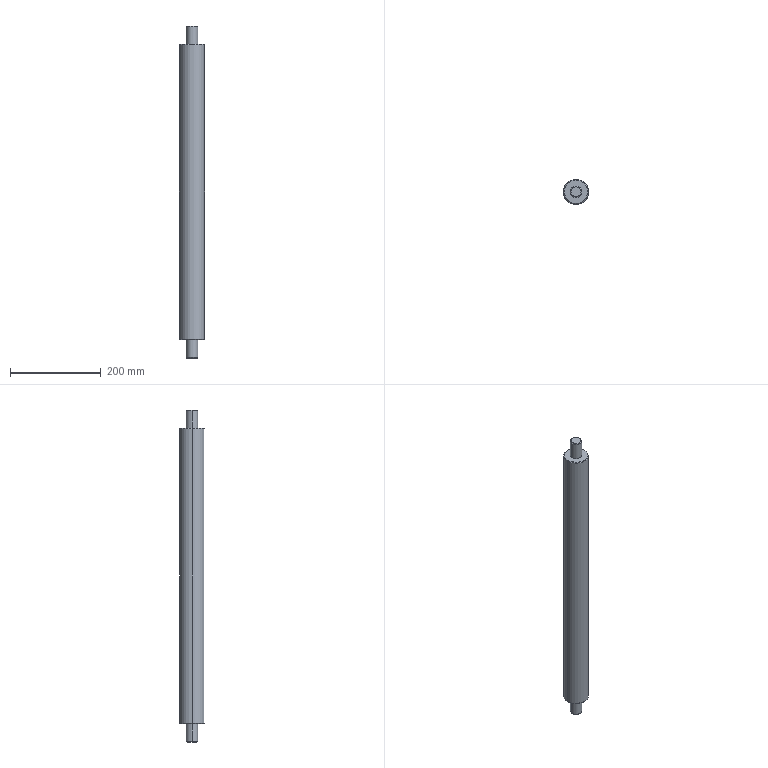Part | SolidWorks | features Chamfer 1, Extrusion 1, ICE 1, MirrorPattern 1 | 1 solid | 18 faces | box 55 x 55 x 730 mm | volume 1583008 mm3 | cone 8 | cylinder 6 | plane 4 | commonest cylinder face diameters 25 x4 55 x2
STEP:
#1=CARTESIAN_POINT('',(26.,0.,325.));
#2=VERTEX_POINT('',#1);
#3=CARTESIAN_POINT('',(-26.,0.,325.));
#4=VERTEX_POINT('',#3);
#5=CARTESIAN_POINT('',(0.,0.,325.));
#6=DIRECTION('',(0.,0.,1.));
#7=DIRECTION('',(1.,0.,0.));
#8=AXIS2_PLACEMENT_3D('',#5,#6,#7);
#9=CIRCLE('',#8,26.);
#10=EDGE_CURVE('',#2,#4,#9,.T.);
#11=ORIENTED_EDGE('',*,*,#10,.F.);
#12=CARTESIAN_POINT('',(27.5,0.,323.5));
#13=VERTEX_POINT('',#12);
#14=CARTESIAN_POINT('',(26.,0.,325.));
#15=DIRECTION('',(0.7071,0.,-0.7071));
#16=VECTOR('',#15,1000.);
#17=LINE('',#14,#16);
#18=EDGE_CURVE('',#2,#13,#17,.T.);
#19=ORIENTED_EDGE('',*,*,#18,.T.);
#20=CARTESIAN_POINT('',(-27.5,0.,323.5));
#21=VERTEX_POINT('',#20);
#22=CARTESIAN_POINT('',(0.,0.,323.5));
#23=DIRECTION('',(0.,0.,-1.));
#24=DIRECTION('',(1.,0.,0.));
#25=AXIS2_PLACEMENT_3D('',#22,#23,#24);
#26=CIRCLE('',#25,27.5);
#27=EDGE_CURVE('',#21,#13,#26,.T.);
#28=ORIENTED_EDGE('',*,*,#27,.F.);
#29=CARTESIAN_POINT('',(-26.,0.,325.));
#30=DIRECTION('',(-0.7071,0.,-0.7071));
#31=VECTOR('',#30,1000.);
#32=LINE('',#29,#31);
#33=EDGE_CURVE('',#4,#21,#32,.T.);
#34=ORIENTED_EDGE('',*,*,#33,.F.);
#35=EDGE_LOOP('',(#11,#19,#28,#34));
#36=FACE_OUTER_BOUND('',#35,.T.);
#37=CARTESIAN_POINT('',(0.,0.,325.));
#38=DIRECTION('',(0.,0.,-1.));
#39=DIRECTION('',(-1.,0.,0.));
#40=AXIS2_PLACEMENT_3D('',#37,#38,#39);
#41=CONICAL_SURFACE('',#40,26.,0.7854);
#42=ADVANCED_FACE('',(#36),#41,.T.);
#43=CARTESIAN_POINT('',(11.,0.,365.));
#44=VERTEX_POINT('',#43);
#45=CARTESIAN_POINT('',(-11.,0.,365.));
#46=VERTEX_POINT('',#45);
#47=CARTESIAN_POINT('',(0.,0.,365.));
#48=DIRECTION('',(0.,0.,1.));
#49=DIRECTION('',(1.,0.,0.));
#50=AXIS2_PLACEMENT_3D('',#47,#48,#49);
#51=CIRCLE('',#50,11.);
#52=EDGE_CURVE('',#44,#46,#51,.T.);
#53=ORIENTED_EDGE('',*,*,#52,.F.);
#54=CARTESIAN_POINT('',(12.5,0.,363.5));
#55=VERTEX_POINT('',#54);
#56=CARTESIAN_POINT('',(11.,0.,365.));
#57=DIRECTION('',(0.7071,0.,-0.7071));
#58=VECTOR('',#57,1000.);
#59=LINE('',#56,#58);
#60=EDGE_CURVE('',#44,#55,#59,.T.);
#61=ORIENTED_EDGE('',*,*,#60,.T.);
#62=CARTESIAN_POINT('',(-12.5,0.,363.5));
#63=VERTEX_POINT('',#62);
#64=CARTESIAN_POINT('',(0.,0.,363.5));
#65=DIRECTION('',(0.,0.,-1.));
#66=DIRECTION('',(1.,0.,0.));
#67=AXIS2_PLACEMENT_3D('',#64,#65,#66);
#68=CIRCLE('',#67,12.5);
#69=EDGE_CURVE('',#63,#55,#68,.T.);
#70=ORIENTED_EDGE('',*,*,#69,.F.);
#71=CARTESIAN_POINT('',(-11.,0.,365.));
#72=DIRECTION('',(-0.7071,0.,-0.7071));
#73=VECTOR('',#72,1000.);
#74=LINE('',#71,#73);
#75=EDGE_CURVE('',#46,#63,#74,.T.);
#76=ORIENTED_EDGE('',*,*,#75,.F.);
#77=EDGE_LOOP('',(#53,#61,#70,#76));
#78=FACE_OUTER_BOUND('',#77,.T.);
#79=CARTESIAN_POINT('',(0.,0.,365.));
#80=DIRECTION('',(0.,0.,-1.));
#81=DIRECTION('',(-1.,0.,0.));
#82=AXIS2_PLACEMENT_3D('',#79,#80,#81);
#83=CONICAL_SURFACE('',#82,11.,0.7854);
#84=ADVANCED_FACE('',(#78),#83,.T.);
#85=CARTESIAN_POINT('',(-26.,0.,-325.));
#86=VERTEX_POINT('',#85);
#87=CARTESIAN_POINT('',(26.,0.,-325.));
#88=VERTEX_POINT('',#87);
#89=CARTESIAN_POINT('',(0.,0.,-325.));
#90=DIRECTION('',(0.,0.,-1.));
#91=DIRECTION('',(1.,0.,0.));
#92=AXIS2_PLACEMENT_3D('',#89,#90,#91);
#93=CIRCLE('',#92,26.);
#94=EDGE_CURVE('',#86,#88,#93,.T.);
#95=ORIENTED_EDGE('',*,*,#94,.F.);
#96=CARTESIAN_POINT('',(-27.5,0.,-323.5));
#97=VERTEX_POINT('',#96);
#98=CARTESIAN_POINT('',(-27.5,0.,-323.5));
#99=DIRECTION('',(-0.7071,0.,0.7071));
#100=VECTOR('',#99,1000.);
#101=LINE('',#98,#100);
#102=EDGE_CURVE('',#86,#97,#101,.T.);
#103=ORIENTED_EDGE('',*,*,#102,.T.);
#104=CARTESIAN_POINT('',(27.5,0.,-323.5));
#105=VERTEX_POINT('',#104);
#106=CARTESIAN_POINT('',(0.,0.,-323.5));
#107=DIRECTION('',(0.,0.,1.));
#108=DIRECTION('',(1.,0.,0.));
#109=AXIS2_PLACEMENT_3D('',#106,#107,#108);
#110=CIRCLE('',#109,27.5);
#111=EDGE_CURVE('',#105,#97,#110,.T.);
#112=ORIENTED_EDGE('',*,*,#111,.F.);
#113=CARTESIAN_POINT('',(27.5,0.,-323.5));
#114=DIRECTION('',(0.7071,0.,0.7071));
#115=VECTOR('',#114,1000.);
#116=LINE('',#113,#115);
#117=EDGE_CURVE('',#88,#105,#116,.T.);
#118=ORIENTED_EDGE('',*,*,#117,.F.);
#119=EDGE_LOOP('',(#95,#103,#112,#118));
#120=FACE_OUTER_BOUND('',#119,.T.);
#121=CARTESIAN_POINT('',(0.,0.,-323.5));
#122=DIRECTION('',(0.,0.,1.));
#123=DIRECTION('',(1.,0.,0.));
#124=AXIS2_PLACEMENT_3D('',#121,#122,#123);
#125=CONICAL_SURFACE('',#124,27.5,0.7854);
#126=ADVANCED_FACE('',(#120),#125,.T.);
#127=CARTESIAN_POINT('',(-11.,0.,-365.));
#128=VERTEX_POINT('',#127);
#129=CARTESIAN_POINT('',(11.,0.,-365.));
#130=VERTEX_POINT('',#129);
#131=CARTESIAN_POINT('',(0.,0.,-365.));
#132=DIRECTION('',(0.,0.,-1.));
#133=DIRECTION('',(-1.,0.,0.));
#134=AXIS2_PLACEMENT_3D('',#131,#132,#133);
#135=CIRCLE('',#134,11.);
#136=EDGE_CURVE('',#128,#130,#135,.T.);
#137=ORIENTED_EDGE('',*,*,#136,.F.);
#138=CARTESIAN_POINT('',(-12.5,0.,-363.5));
#139=VERTEX_POINT('',#138);
#140=CARTESIAN_POINT('',(-12.5,0.,-363.5));
#141=DIRECTION('',(-0.7071,0.,0.7071));
#142=VECTOR('',#141,1000.);
#143=LINE('',#140,#142);
#144=EDGE_CURVE('',#128,#139,#143,.T.);
#145=ORIENTED_EDGE('',*,*,#144,.T.);
#146=CARTESIAN_POINT('',(12.5,0.,-363.5));
#147=VERTEX_POINT('',#146);
#148=CARTESIAN_POINT('',(0.,0.,-363.5));
#149=DIRECTION('',(0.,0.,1.));
#150=DIRECTION('',(-1.,0.,0.));
#151=AXIS2_PLACEMENT_3D('',#148,#149,#150);
#152=CIRCLE('',#151,12.5);
#153=EDGE_CURVE('',#147,#139,#152,.T.);
#154=ORIENTED_EDGE('',*,*,#153,.F.);
#155=CARTESIAN_POINT('',(12.5,0.,-363.5));
#156=DIRECTION('',(0.7071,0.,0.7071));
#157=VECTOR('',#156,1000.);
#158=LINE('',#155,#157);
#159=EDGE_CURVE('',#130,#147,#158,.T.);
#160=ORIENTED_EDGE('',*,*,#159,.F.);
#161=EDGE_LOOP('',(#137,#145,#154,#160));
#162=FACE_OUTER_BOUND('',#161,.T.);
#163=CARTESIAN_POINT('',(0.,0.,-363.5));
#164=DIRECTION('',(0.,0.,1.));
#165=DIRECTION('',(1.,0.,0.));
#166=AXIS2_PLACEMENT_3D('',#163,#164,#165);
#167=CONICAL_SURFACE('',#166,12.5,0.7854);
#168=ADVANCED_FACE('',(#162),#167,.T.);
#169=ORIENTED_EDGE('',*,*,#153,.T.);
#170=CARTESIAN_POINT('',(-12.5,0.,-325.));
#171=VERTEX_POINT('',#170);
#172=CARTESIAN_POINT('',(-12.5,0.,-365.));
#173=DIRECTION('',(0.,0.,1.));
#174=VECTOR('',#173,1000.);
#175=LINE('',#172,#174);
#176=EDGE_CURVE('',#139,#171,#175,.T.);
#177=ORIENTED_EDGE('',*,*,#176,.T.);
#178=CARTESIAN_POINT('',(12.5,0.,-325.));
#179=VERTEX_POINT('',#178);
#180=CARTESIAN_POINT('',(0.,0.,-325.));
#181=DIRECTION('',(0.,0.,1.));
#182=DIRECTION('',(1.,0.,0.));
#183=AXIS2_PLACEMENT_3D('',#180,#181,#182);
#184=CIRCLE('',#183,12.5);
#185=EDGE_CURVE('',#179,#171,#184,.T.);
#186=ORIENTED_EDGE('',*,*,#185,.F.);
#187=CARTESIAN_POINT('',(12.5,0.,-365.));
#188=DIRECTION('',(0.,0.,1.));
#189=VECTOR('',#188,1000.);
#190=LINE('',#187,#189);
#191=EDGE_CURVE('',#147,#179,#190,.T.);
#192=ORIENTED_EDGE('',*,*,#191,.F.);
#193=EDGE_LOOP('',(#169,#177,#186,#192));
#194=FACE_OUTER_BOUND('',#193,.T.);
#195=CARTESIAN_POINT('',(0.,0.,-365.));
#196=DIRECTION('',(0.,0.,1.));
#197=DIRECTION('',(1.,0.,0.));
#198=AXIS2_PLACEMENT_3D('',#195,#196,#197);
#199=CYLINDRICAL_SURFACE('',#198,12.5);
#200=ADVANCED_FACE('',(#194),#199,.T.);
#201=ORIENTED_EDGE('',*,*,#69,.T.);
#202=CARTESIAN_POINT('',(12.5,0.,325.));
#203=VERTEX_POINT('',#202);
#204=CARTESIAN_POINT('',(12.5,0.,365.));
#205=DIRECTION('',(0.,0.,-1.));
#206=VECTOR('',#205,1000.);
#207=LINE('',#204,#206);
#208=EDGE_CURVE('',#55,#203,#207,.T.);
#209=ORIENTED_EDGE('',*,*,#208,.T.);
#210=CARTESIAN_POINT('',(-12.5,0.,325.));
#211=VERTEX_POINT('',#210);
#212=CARTESIAN_POINT('',(0.,0.,325.));
#213=DIRECTION('',(0.,0.,1.));
#214=DIRECTION('',(1.,0.,0.));
#215=AXIS2_PLACEMENT_3D('',#212,#213,#214);
#216=CIRCLE('',#215,12.5);
#217=EDGE_CURVE('',#203,#211,#216,.T.);
#218=ORIENTED_EDGE('',*,*,#217,.T.);
#219=CARTESIAN_POINT('',(-12.5,0.,365.));
#220=DIRECTION('',(0.,0.,-1.));
#221=VECTOR('',#220,1000.);
#222=LINE('',#219,#221);
#223=EDGE_CURVE('',#63,#211,#222,.T.);
#224=ORIENTED_EDGE('',*,*,#223,.F.);
#225=EDGE_LOOP('',(#201,#209,#218,#224));
#226=FACE_OUTER_BOUND('',#225,.T.);
#227=CARTESIAN_POINT('',(0.,0.,365.));
#228=DIRECTION('',(0.,0.,-1.));
#229=DIRECTION('',(-1.,0.,0.));
#230=AXIS2_PLACEMENT_3D('',#227,#228,#229);
#231=CYLINDRICAL_SURFACE('',#230,12.5);
#232=ADVANCED_FACE('',(#226),#231,.T.);
#233=ORIENTED_EDGE('',*,*,#27,.T.);
#234=CARTESIAN_POINT('',(27.5,0.,325.));
#235=DIRECTION('',(0.,0.,-1.));
#236=VECTOR('',#235,1000.);
#237=LINE('',#234,#236);
#238=EDGE_CURVE('',#13,#105,#237,.T.);
#239=ORIENTED_EDGE('',*,*,#238,.T.);
#240=ORIENTED_EDGE('',*,*,#111,.T.);
#241=CARTESIAN_POINT('',(-27.5,0.,325.));
#242=DIRECTION('',(0.,0.,-1.));
#243=VECTOR('',#242,1000.);
#244=LINE('',#241,#243);
#245=EDGE_CURVE('',#21,#97,#244,.T.);
#246=ORIENTED_EDGE('',*,*,#245,.F.);
#247=EDGE_LOOP('',(#233,#239,#240,#246));
#248=FACE_OUTER_BOUND('',#247,.T.);
#249=CARTESIAN_POINT('',(0.,0.,325.));
#250=DIRECTION('',(0.,0.,-1.));
#251=DIRECTION('',(-1.,0.,0.));
#252=AXIS2_PLACEMENT_3D('',#249,#250,#251);
#253=CYLINDRICAL_SURFACE('',#252,27.5);
#254=ADVANCED_FACE('',(#248),#253,.T.);
#255=ORIENTED_EDGE('',*,*,#238,.F.);
#256=CARTESIAN_POINT('',(0.,0.,323.5));
#257=DIRECTION('',(0.,0.,-1.));
#258=DIRECTION('',(1.,0.,0.));
#259=AXIS2_PLACEMENT_3D('',#256,#257,#258);
#260=CIRCLE('',#259,27.5);
#261=EDGE_CURVE('',#13,#21,#260,.T.);
#262=ORIENTED_EDGE('',*,*,#261,.T.);
#263=ORIENTED_EDGE('',*,*,#245,.T.);
#264=CARTESIAN_POINT('',(0.,0.,-323.5));
#265=DIRECTION('',(0.,0.,1.));
#266=DIRECTION('',(1.,0.,0.));
#267=AXIS2_PLACEMENT_3D('',#264,#265,#266);
#268=CIRCLE('',#267,27.5);
#269=EDGE_CURVE('',#97,#105,#268,.T.);
#270=ORIENTED_EDGE('',*,*,#269,.T.);
#271=EDGE_LOOP('',(#255,#262,#263,#270));
#272=FACE_OUTER_BOUND('',#271,.T.);
#273=CARTESIAN_POINT('',(0.,0.,325.));
#274=DIRECTION('',(0.,0.,-1.));
#275=DIRECTION('',(-1.,0.,0.));
#276=AXIS2_PLACEMENT_3D('',#273,#274,#275);
#277=CYLINDRICAL_SURFACE('',#276,27.5);
#278=ADVANCED_FACE('',(#272),#277,.T.);
#279=CARTESIAN_POINT('',(0.,0.,325.));
#280=DIRECTION('',(0.,0.,1.));
#281=DIRECTION('',(1.,0.,0.));
#282=AXIS2_PLACEMENT_3D('',#279,#280,#281);
#283=CIRCLE('',#282,26.);
#284=EDGE_CURVE('',#4,#2,#283,.T.);
#285=ORIENTED_EDGE('',*,*,#284,.T.);
#286=ORIENTED_EDGE('',*,*,#10,.T.);
#287=EDGE_LOOP('',(#285,#286));
#288=FACE_OUTER_BOUND('',#287,.T.);
#289=CARTESIAN_POINT('',(0.,0.,325.));
#290=DIRECTION('',(0.,0.,1.));
#291=DIRECTION('',(1.,0.,0.));
#292=AXIS2_PLACEMENT_3D('',#289,#290,#291);
#293=CIRCLE('',#292,12.5);
#294=EDGE_CURVE('',#211,#203,#293,.T.);
#295=ORIENTED_EDGE('',*,*,#294,.F.);
#296=ORIENTED_EDGE('',*,*,#217,.F.);
#297=EDGE_LOOP('',(#295,#296));
#298=FACE_BOUND('',#297,.T.);
#299=CARTESIAN_POINT('',(0.,0.,325.));
#300=DIRECTION('',(0.,0.,1.));
#301=DIRECTION('',(1.,0.,0.));
#302=AXIS2_PLACEMENT_3D('',#299,#300,#301);
#303=PLANE('',#302);
#304=ADVANCED_FACE('',(#288,#298),#303,.T.);
#305=CARTESIAN_POINT('',(0.,0.,-325.));
#306=DIRECTION('',(0.,0.,-1.));
#307=DIRECTION('',(1.,0.,0.));
#308=AXIS2_PLACEMENT_3D('',#305,#306,#307);
#309=CIRCLE('',#308,26.);
#310=EDGE_CURVE('',#88,#86,#309,.T.);
#311=ORIENTED_EDGE('',*,*,#310,.T.);
#312=ORIENTED_EDGE('',*,*,#94,.T.);
#313=EDGE_LOOP('',(#311,#312));
#314=FACE_OUTER_BOUND('',#313,.T.);
#315=ORIENTED_EDGE('',*,*,#185,.T.);
#316=CARTESIAN_POINT('',(0.,0.,-325.));
#317=DIRECTION('',(0.,0.,1.));
#318=DIRECTION('',(1.,0.,0.));
#319=AXIS2_PLACEMENT_3D('',#316,#317,#318);
#320=CIRCLE('',#319,12.5);
#321=EDGE_CURVE('',#171,#179,#320,.T.);
#322=ORIENTED_EDGE('',*,*,#321,.T.);
#323=EDGE_LOOP('',(#315,#322));
#324=FACE_BOUND('',#323,.T.);
#325=CARTESIAN_POINT('',(0.,0.,-325.));
#326=DIRECTION('',(0.,0.,1.));
#327=DIRECTION('',(1.,0.,0.));
#328=AXIS2_PLACEMENT_3D('',#325,#326,#327);
#329=PLANE('',#328);
#330=ADVANCED_FACE('',(#314,#324),#329,.F.);
#331=ORIENTED_EDGE('',*,*,#208,.F.);
#332=CARTESIAN_POINT('',(0.,0.,363.5));
#333=DIRECTION('',(0.,0.,-1.));
#334=DIRECTION('',(1.,0.,0.));
#335=AXIS2_PLACEMENT_3D('',#332,#333,#334);
#336=CIRCLE('',#335,12.5);
#337=EDGE_CURVE('',#55,#63,#336,.T.);
#338=ORIENTED_EDGE('',*,*,#337,.T.);
#339=ORIENTED_EDGE('',*,*,#223,.T.);
#340=ORIENTED_EDGE('',*,*,#294,.T.);
#341=EDGE_LOOP('',(#331,#338,#339,#340));
#342=FACE_OUTER_BOUND('',#341,.T.);
#343=CARTESIAN_POINT('',(0.,0.,365.));
#344=DIRECTION('',(0.,0.,-1.));
#345=DIRECTION('',(-1.,0.,0.));
#346=AXIS2_PLACEMENT_3D('',#343,#344,#345);
#347=CYLINDRICAL_SURFACE('',#346,12.5);
#348=ADVANCED_FACE('',(#342),#347,.T.);
#349=CARTESIAN_POINT('',(0.,0.,365.));
#350=DIRECTION('',(0.,0.,1.));
#351=DIRECTION('',(1.,0.,0.));
#352=AXIS2_PLACEMENT_3D('',#349,#350,#351);
#353=CIRCLE('',#352,11.);
#354=EDGE_CURVE('',#46,#44,#353,.T.);
#355=ORIENTED_EDGE('',*,*,#354,.T.);
#356=ORIENTED_EDGE('',*,*,#52,.T.);
#357=EDGE_LOOP('',(#355,#356));
#358=FACE_OUTER_BOUND('',#357,.T.);
#359=CARTESIAN_POINT('',(0.,0.,365.));
#360=DIRECTION('',(0.,0.,1.));
#361=DIRECTION('',(1.,0.,0.));
#362=AXIS2_PLACEMENT_3D('',#359,#360,#361);
#363=PLANE('',#362);
#364=ADVANCED_FACE('',(#358),#363,.T.);
#365=ORIENTED_EDGE('',*,*,#176,.F.);
#366=CARTESIAN_POINT('',(0.,0.,-363.5));
#367=DIRECTION('',(0.,0.,1.));
#368=DIRECTION('',(-1.,0.,0.));
#369=AXIS2_PLACEMENT_3D('',#366,#367,#368);
#370=CIRCLE('',#369,12.5);
#371=EDGE_CURVE('',#139,#147,#370,.T.);
#372=ORIENTED_EDGE('',*,*,#371,.T.);
#373=ORIENTED_EDGE('',*,*,#191,.T.);
#374=ORIENTED_EDGE('',*,*,#321,.F.);
#375=EDGE_LOOP('',(#365,#372,#373,#374));
#376=FACE_OUTER_BOUND('',#375,.T.);
#377=CARTESIAN_POINT('',(0.,0.,-365.));
#378=DIRECTION('',(0.,0.,1.));
#379=DIRECTION('',(1.,0.,0.));
#380=AXIS2_PLACEMENT_3D('',#377,#378,#379);
#381=CYLINDRICAL_SURFACE('',#380,12.5);
#382=ADVANCED_FACE('',(#376),#381,.T.);
#383=CARTESIAN_POINT('',(0.,0.,-365.));
#384=DIRECTION('',(0.,0.,-1.));
#385=DIRECTION('',(-1.,0.,0.));
#386=AXIS2_PLACEMENT_3D('',#383,#384,#385);
#387=CIRCLE('',#386,11.);
#388=EDGE_CURVE('',#130,#128,#387,.T.);
#389=ORIENTED_EDGE('',*,*,#388,.T.);
#390=ORIENTED_EDGE('',*,*,#136,.T.);
#391=EDGE_LOOP('',(#389,#390));
#392=FACE_OUTER_BOUND('',#391,.T.);
#393=CARTESIAN_POINT('',(0.,0.,-365.));
#394=DIRECTION('',(0.,0.,-1.));
#395=DIRECTION('',(1.,0.,0.));
#396=AXIS2_PLACEMENT_3D('',#393,#394,#395);
#397=PLANE('',#396);
#398=ADVANCED_FACE('',(#392),#397,.T.);
#399=ORIENTED_EDGE('',*,*,#144,.F.);
#400=ORIENTED_EDGE('',*,*,#388,.F.);
#401=ORIENTED_EDGE('',*,*,#159,.T.);
#402=ORIENTED_EDGE('',*,*,#371,.F.);
#403=EDGE_LOOP('',(#399,#400,#401,#402));
#404=FACE_OUTER_BOUND('',#403,.T.);
#405=CARTESIAN_POINT('',(0.,0.,-363.5));
#406=DIRECTION('',(0.,0.,1.));
#407=DIRECTION('',(1.,0.,0.));
#408=AXIS2_PLACEMENT_3D('',#405,#406,#407);
#409=CONICAL_SURFACE('',#408,12.5,0.7854);
#410=ADVANCED_FACE('',(#404),#409,.T.);
#411=ORIENTED_EDGE('',*,*,#102,.F.);
#412=ORIENTED_EDGE('',*,*,#310,.F.);
#413=ORIENTED_EDGE('',*,*,#117,.T.);
#414=ORIENTED_EDGE('',*,*,#269,.F.);
#415=EDGE_LOOP('',(#411,#412,#413,#414));
#416=FACE_OUTER_BOUND('',#415,.T.);
#417=CARTESIAN_POINT('',(0.,0.,-323.5));
#418=DIRECTION('',(0.,0.,1.));
#419=DIRECTION('',(1.,0.,0.));
#420=AXIS2_PLACEMENT_3D('',#417,#418,#419);
#421=CONICAL_SURFACE('',#420,27.5,0.7854);
#422=ADVANCED_FACE('',(#416),#421,.T.);
#423=ORIENTED_EDGE('',*,*,#60,.F.);
#424=ORIENTED_EDGE('',*,*,#354,.F.);
#425=ORIENTED_EDGE('',*,*,#75,.T.);
#426=ORIENTED_EDGE('',*,*,#337,.F.);
#427=EDGE_LOOP('',(#423,#424,#425,#426));
#428=FACE_OUTER_BOUND('',#427,.T.);
#429=CARTESIAN_POINT('',(0.,0.,365.));
#430=DIRECTION('',(0.,0.,-1.));
#431=DIRECTION('',(-1.,0.,0.));
#432=AXIS2_PLACEMENT_3D('',#429,#430,#431);
#433=CONICAL_SURFACE('',#432,11.,0.7854);
#434=ADVANCED_FACE('',(#428),#433,.T.);
#435=ORIENTED_EDGE('',*,*,#18,.F.);
#436=ORIENTED_EDGE('',*,*,#284,.F.);
#437=ORIENTED_EDGE('',*,*,#33,.T.);
#438=ORIENTED_EDGE('',*,*,#261,.F.);
#439=EDGE_LOOP('',(#435,#436,#437,#438));
#440=FACE_OUTER_BOUND('',#439,.T.);
#441=CARTESIAN_POINT('',(0.,0.,325.));
#442=DIRECTION('',(0.,0.,-1.));
#443=DIRECTION('',(-1.,0.,0.));
#444=AXIS2_PLACEMENT_3D('',#441,#442,#443);
#445=CONICAL_SURFACE('',#444,26.,0.7854);
#446=ADVANCED_FACE('',(#440),#445,.T.);
#447=CLOSED_SHELL('',(#42,#84,#126,#168,#200,#232,#254,#278,#304,#330,#348,#364,#382,#398,#410,#422,#434,#446));
#448=MANIFOLD_SOLID_BREP('',#447);
#449=CARTESIAN_POINT('',(0.,0.,0.));
#450=DIRECTION('',(0.,0.,1.));
#451=DIRECTION('',(1.,0.,0.));
#452=AXIS2_PLACEMENT_3D('',#449,#450,#451);
#453=(LENGTH_UNIT()NAMED_UNIT(*)SI_UNIT(.MILLI.,.METRE.));
#454=UNCERTAINTY_MEASURE_WITH_UNIT(LENGTH_MEASURE(0.00001),#453,'','');
#455=(NAMED_UNIT(*)PLANE_ANGLE_UNIT()SI_UNIT($,.RADIAN.));
#456=(NAMED_UNIT(*)SI_UNIT($,.STERADIAN.)SOLID_ANGLE_UNIT());
#457=(GEOMETRIC_REPRESENTATION_CONTEXT(3)GLOBAL_UNCERTAINTY_ASSIGNED_CONTEXT((#454))GLOBAL_UNIT_ASSIGNED_CONTEXT((#453,#455,#456))REPRESENTATION_CONTEXT('',''));
#458=ADVANCED_BREP_SHAPE_REPRESENTATION('',(#448,#452),#457);